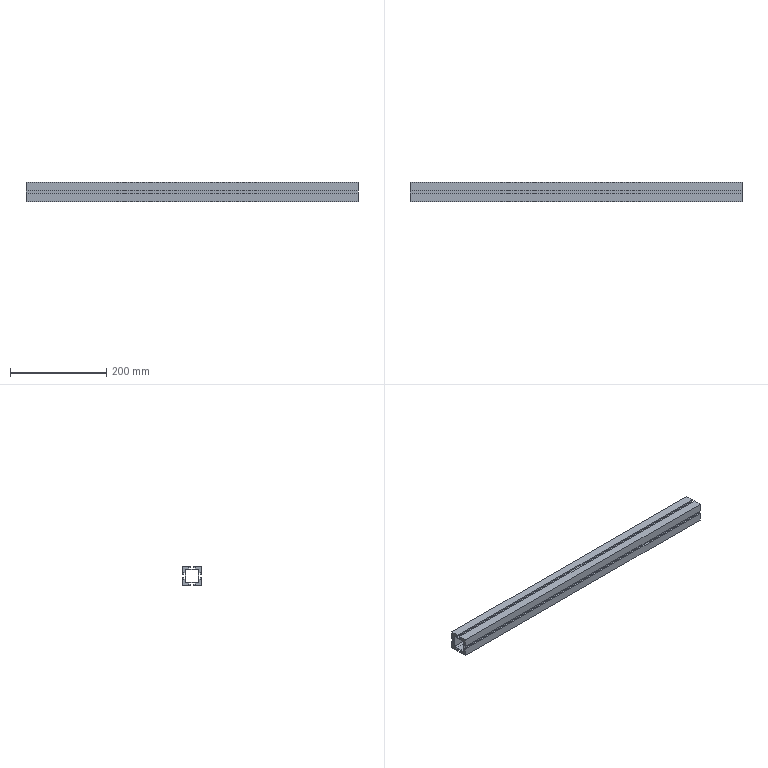Part | SolidWorks | features Extrusion 1 | 1 solid | 42 faces | box 690 x 40 x 40 mm | volume 480240 mm3 | plane 42
STEP:
#1=CARTESIAN_POINT('',(690.,3.,-20.));
#2=VERTEX_POINT('',#1);
#3=CARTESIAN_POINT('',(690.,20.,-20.));
#4=VERTEX_POINT('',#3);
#5=CARTESIAN_POINT('',(690.,3.,-20.));
#6=DIRECTION('',(0.,1.,0.));
#7=VECTOR('',#6,1000.);
#8=LINE('',#5,#7);
#9=EDGE_CURVE('',#2,#4,#8,.T.);
#10=ORIENTED_EDGE('',*,*,#9,.T.);
#11=CARTESIAN_POINT('',(690.,20.,-3.));
#12=VERTEX_POINT('',#11);
#13=CARTESIAN_POINT('',(690.,20.,-3.));
#14=DIRECTION('',(0.,0.,1.));
#15=VECTOR('',#14,1000.);
#16=LINE('',#13,#15);
#17=EDGE_CURVE('',#4,#12,#16,.T.);
#18=ORIENTED_EDGE('',*,*,#17,.T.);
#19=CARTESIAN_POINT('',(690.,17.,-3.));
#20=VERTEX_POINT('',#19);
#21=CARTESIAN_POINT('',(690.,20.,-3.));
#22=DIRECTION('',(0.,-1.,0.));
#23=VECTOR('',#22,1000.);
#24=LINE('',#21,#23);
#25=EDGE_CURVE('',#12,#20,#24,.T.);
#26=ORIENTED_EDGE('',*,*,#25,.T.);
#27=CARTESIAN_POINT('',(690.,17.,-6.5));
#28=VERTEX_POINT('',#27);
#29=CARTESIAN_POINT('',(690.,17.,-3.));
#30=DIRECTION('',(0.,0.,-1.));
#31=VECTOR('',#30,1000.);
#32=LINE('',#29,#31);
#33=EDGE_CURVE('',#20,#28,#32,.T.);
#34=ORIENTED_EDGE('',*,*,#33,.T.);
#35=CARTESIAN_POINT('',(690.,14.,-6.5));
#36=VERTEX_POINT('',#35);
#37=CARTESIAN_POINT('',(690.,17.,-6.5));
#38=DIRECTION('',(0.,-1.,0.));
#39=VECTOR('',#38,1000.);
#40=LINE('',#37,#39);
#41=EDGE_CURVE('',#28,#36,#40,.T.);
#42=ORIENTED_EDGE('',*,*,#41,.T.);
#43=CARTESIAN_POINT('',(690.,14.,6.5));
#44=VERTEX_POINT('',#43);
#45=CARTESIAN_POINT('',(690.,14.,6.5));
#46=DIRECTION('',(0.,0.,1.));
#47=VECTOR('',#46,1000.);
#48=LINE('',#45,#47);
#49=EDGE_CURVE('',#36,#44,#48,.T.);
#50=ORIENTED_EDGE('',*,*,#49,.T.);
#51=CARTESIAN_POINT('',(690.,17.,6.5));
#52=VERTEX_POINT('',#51);
#53=CARTESIAN_POINT('',(690.,17.,6.5));
#54=DIRECTION('',(0.,1.,0.));
#55=VECTOR('',#54,1000.);
#56=LINE('',#53,#55);
#57=EDGE_CURVE('',#44,#52,#56,.T.);
#58=ORIENTED_EDGE('',*,*,#57,.T.);
#59=CARTESIAN_POINT('',(690.,17.,3.));
#60=VERTEX_POINT('',#59);
#61=CARTESIAN_POINT('',(690.,17.,6.5));
#62=DIRECTION('',(0.,0.,-1.));
#63=VECTOR('',#62,1000.);
#64=LINE('',#61,#63);
#65=EDGE_CURVE('',#52,#60,#64,.T.);
#66=ORIENTED_EDGE('',*,*,#65,.T.);
#67=CARTESIAN_POINT('',(690.,20.,3.));
#68=VERTEX_POINT('',#67);
#69=CARTESIAN_POINT('',(690.,20.,3.));
#70=DIRECTION('',(0.,1.,0.));
#71=VECTOR('',#70,1000.);
#72=LINE('',#69,#71);
#73=EDGE_CURVE('',#60,#68,#72,.T.);
#74=ORIENTED_EDGE('',*,*,#73,.T.);
#75=CARTESIAN_POINT('',(690.,20.,20.));
#76=VERTEX_POINT('',#75);
#77=CARTESIAN_POINT('',(690.,20.,20.));
#78=DIRECTION('',(0.,0.,1.));
#79=VECTOR('',#78,1000.);
#80=LINE('',#77,#79);
#81=EDGE_CURVE('',#68,#76,#80,.T.);
#82=ORIENTED_EDGE('',*,*,#81,.T.);
#83=CARTESIAN_POINT('',(690.,3.,20.));
#84=VERTEX_POINT('',#83);
#85=CARTESIAN_POINT('',(690.,3.,20.));
#86=DIRECTION('',(0.,-1.,0.));
#87=VECTOR('',#86,1000.);
#88=LINE('',#85,#87);
#89=EDGE_CURVE('',#76,#84,#88,.T.);
#90=ORIENTED_EDGE('',*,*,#89,.T.);
#91=CARTESIAN_POINT('',(690.,3.,17.));
#92=VERTEX_POINT('',#91);
#93=CARTESIAN_POINT('',(690.,3.,17.));
#94=DIRECTION('',(0.,0.,-1.));
#95=VECTOR('',#94,1000.);
#96=LINE('',#93,#95);
#97=EDGE_CURVE('',#84,#92,#96,.T.);
#98=ORIENTED_EDGE('',*,*,#97,.T.);
#99=CARTESIAN_POINT('',(690.,6.5,17.));
#100=VERTEX_POINT('',#99);
#101=CARTESIAN_POINT('',(690.,3.,17.));
#102=DIRECTION('',(0.,1.,0.));
#103=VECTOR('',#102,1000.);
#104=LINE('',#101,#103);
#105=EDGE_CURVE('',#92,#100,#104,.T.);
#106=ORIENTED_EDGE('',*,*,#105,.T.);
#107=CARTESIAN_POINT('',(690.,6.5,14.));
#108=VERTEX_POINT('',#107);
#109=CARTESIAN_POINT('',(690.,6.5,14.));
#110=DIRECTION('',(0.,0.,-1.));
#111=VECTOR('',#110,1000.);
#112=LINE('',#109,#111);
#113=EDGE_CURVE('',#100,#108,#112,.T.);
#114=ORIENTED_EDGE('',*,*,#113,.T.);
#115=CARTESIAN_POINT('',(690.,-6.5,14.));
#116=VERTEX_POINT('',#115);
#117=CARTESIAN_POINT('',(690.,-6.5,14.));
#118=DIRECTION('',(0.,-1.,0.));
#119=VECTOR('',#118,1000.);
#120=LINE('',#117,#119);
#121=EDGE_CURVE('',#108,#116,#120,.T.);
#122=ORIENTED_EDGE('',*,*,#121,.T.);
#123=CARTESIAN_POINT('',(690.,-6.5,17.));
#124=VERTEX_POINT('',#123);
#125=CARTESIAN_POINT('',(690.,-6.5,14.));
#126=DIRECTION('',(0.,0.,1.));
#127=VECTOR('',#126,1000.);
#128=LINE('',#125,#127);
#129=EDGE_CURVE('',#116,#124,#128,.T.);
#130=ORIENTED_EDGE('',*,*,#129,.T.);
#131=CARTESIAN_POINT('',(690.,-3.,17.));
#132=VERTEX_POINT('',#131);
#133=CARTESIAN_POINT('',(690.,-6.5,17.));
#134=DIRECTION('',(0.,1.,0.));
#135=VECTOR('',#134,1000.);
#136=LINE('',#133,#135);
#137=EDGE_CURVE('',#124,#132,#136,.T.);
#138=ORIENTED_EDGE('',*,*,#137,.T.);
#139=CARTESIAN_POINT('',(690.,-3.,20.));
#140=VERTEX_POINT('',#139);
#141=CARTESIAN_POINT('',(690.,-3.,17.));
#142=DIRECTION('',(0.,0.,1.));
#143=VECTOR('',#142,1000.);
#144=LINE('',#141,#143);
#145=EDGE_CURVE('',#132,#140,#144,.T.);
#146=ORIENTED_EDGE('',*,*,#145,.T.);
#147=CARTESIAN_POINT('',(690.,-20.,20.));
#148=VERTEX_POINT('',#147);
#149=CARTESIAN_POINT('',(690.,-20.,20.));
#150=DIRECTION('',(0.,-1.,0.));
#151=VECTOR('',#150,1000.);
#152=LINE('',#149,#151);
#153=EDGE_CURVE('',#140,#148,#152,.T.);
#154=ORIENTED_EDGE('',*,*,#153,.T.);
#155=CARTESIAN_POINT('',(690.,-20.,3.));
#156=VERTEX_POINT('',#155);
#157=CARTESIAN_POINT('',(690.,-20.,20.));
#158=DIRECTION('',(0.,0.,-1.));
#159=VECTOR('',#158,1000.);
#160=LINE('',#157,#159);
#161=EDGE_CURVE('',#148,#156,#160,.T.);
#162=ORIENTED_EDGE('',*,*,#161,.T.);
#163=CARTESIAN_POINT('',(690.,-17.,3.));
#164=VERTEX_POINT('',#163);
#165=CARTESIAN_POINT('',(690.,-20.,3.));
#166=DIRECTION('',(0.,1.,0.));
#167=VECTOR('',#166,1000.);
#168=LINE('',#165,#167);
#169=EDGE_CURVE('',#156,#164,#168,.T.);
#170=ORIENTED_EDGE('',*,*,#169,.T.);
#171=CARTESIAN_POINT('',(690.,-17.,6.5));
#172=VERTEX_POINT('',#171);
#173=CARTESIAN_POINT('',(690.,-17.,6.5));
#174=DIRECTION('',(0.,0.,1.));
#175=VECTOR('',#174,1000.);
#176=LINE('',#173,#175);
#177=EDGE_CURVE('',#164,#172,#176,.T.);
#178=ORIENTED_EDGE('',*,*,#177,.T.);
#179=CARTESIAN_POINT('',(690.,-14.,6.5));
#180=VERTEX_POINT('',#179);
#181=CARTESIAN_POINT('',(690.,-17.,6.5));
#182=DIRECTION('',(0.,1.,0.));
#183=VECTOR('',#182,1000.);
#184=LINE('',#181,#183);
#185=EDGE_CURVE('',#172,#180,#184,.T.);
#186=ORIENTED_EDGE('',*,*,#185,.T.);
#187=CARTESIAN_POINT('',(690.,-14.,-6.5));
#188=VERTEX_POINT('',#187);
#189=CARTESIAN_POINT('',(690.,-14.,6.5));
#190=DIRECTION('',(0.,0.,-1.));
#191=VECTOR('',#190,1000.);
#192=LINE('',#189,#191);
#193=EDGE_CURVE('',#180,#188,#192,.T.);
#194=ORIENTED_EDGE('',*,*,#193,.T.);
#195=CARTESIAN_POINT('',(690.,-17.,-6.5));
#196=VERTEX_POINT('',#195);
#197=CARTESIAN_POINT('',(690.,-17.,-6.5));
#198=DIRECTION('',(0.,-1.,0.));
#199=VECTOR('',#198,1000.);
#200=LINE('',#197,#199);
#201=EDGE_CURVE('',#188,#196,#200,.T.);
#202=ORIENTED_EDGE('',*,*,#201,.T.);
#203=CARTESIAN_POINT('',(690.,-17.,-3.));
#204=VERTEX_POINT('',#203);
#205=CARTESIAN_POINT('',(690.,-17.,-3.));
#206=DIRECTION('',(0.,0.,1.));
#207=VECTOR('',#206,1000.);
#208=LINE('',#205,#207);
#209=EDGE_CURVE('',#196,#204,#208,.T.);
#210=ORIENTED_EDGE('',*,*,#209,.T.);
#211=CARTESIAN_POINT('',(690.,-20.,-3.));
#212=VERTEX_POINT('',#211);
#213=CARTESIAN_POINT('',(690.,-20.,-3.));
#214=DIRECTION('',(0.,-1.,0.));
#215=VECTOR('',#214,1000.);
#216=LINE('',#213,#215);
#217=EDGE_CURVE('',#204,#212,#216,.T.);
#218=ORIENTED_EDGE('',*,*,#217,.T.);
#219=CARTESIAN_POINT('',(690.,-20.,-20.));
#220=VERTEX_POINT('',#219);
#221=CARTESIAN_POINT('',(690.,-20.,-3.));
#222=DIRECTION('',(0.,0.,-1.));
#223=VECTOR('',#222,1000.);
#224=LINE('',#221,#223);
#225=EDGE_CURVE('',#212,#220,#224,.T.);
#226=ORIENTED_EDGE('',*,*,#225,.T.);
#227=CARTESIAN_POINT('',(690.,-3.,-20.));
#228=VERTEX_POINT('',#227);
#229=CARTESIAN_POINT('',(690.,-20.,-20.));
#230=DIRECTION('',(0.,1.,0.));
#231=VECTOR('',#230,1000.);
#232=LINE('',#229,#231);
#233=EDGE_CURVE('',#220,#228,#232,.T.);
#234=ORIENTED_EDGE('',*,*,#233,.T.);
#235=CARTESIAN_POINT('',(690.,-3.,-17.));
#236=VERTEX_POINT('',#235);
#237=CARTESIAN_POINT('',(690.,-3.,-17.));
#238=DIRECTION('',(0.,0.,1.));
#239=VECTOR('',#238,1000.);
#240=LINE('',#237,#239);
#241=EDGE_CURVE('',#228,#236,#240,.T.);
#242=ORIENTED_EDGE('',*,*,#241,.T.);
#243=CARTESIAN_POINT('',(690.,-6.5,-17.));
#244=VERTEX_POINT('',#243);
#245=CARTESIAN_POINT('',(690.,-6.5,-17.));
#246=DIRECTION('',(0.,-1.,0.));
#247=VECTOR('',#246,1000.);
#248=LINE('',#245,#247);
#249=EDGE_CURVE('',#236,#244,#248,.T.);
#250=ORIENTED_EDGE('',*,*,#249,.T.);
#251=CARTESIAN_POINT('',(690.,-6.5,-14.));
#252=VERTEX_POINT('',#251);
#253=CARTESIAN_POINT('',(690.,-6.5,-14.));
#254=DIRECTION('',(0.,0.,1.));
#255=VECTOR('',#254,1000.);
#256=LINE('',#253,#255);
#257=EDGE_CURVE('',#244,#252,#256,.T.);
#258=ORIENTED_EDGE('',*,*,#257,.T.);
#259=CARTESIAN_POINT('',(690.,6.5,-14.));
#260=VERTEX_POINT('',#259);
#261=CARTESIAN_POINT('',(690.,-6.5,-14.));
#262=DIRECTION('',(0.,1.,0.));
#263=VECTOR('',#262,1000.);
#264=LINE('',#261,#263);
#265=EDGE_CURVE('',#252,#260,#264,.T.);
#266=ORIENTED_EDGE('',*,*,#265,.T.);
#267=CARTESIAN_POINT('',(690.,6.5,-17.));
#268=VERTEX_POINT('',#267);
#269=CARTESIAN_POINT('',(690.,6.5,-14.));
#270=DIRECTION('',(0.,0.,-1.));
#271=VECTOR('',#270,1000.);
#272=LINE('',#269,#271);
#273=EDGE_CURVE('',#260,#268,#272,.T.);
#274=ORIENTED_EDGE('',*,*,#273,.T.);
#275=CARTESIAN_POINT('',(690.,3.,-17.));
#276=VERTEX_POINT('',#275);
#277=CARTESIAN_POINT('',(690.,3.,-17.));
#278=DIRECTION('',(0.,-1.,0.));
#279=VECTOR('',#278,1000.);
#280=LINE('',#277,#279);
#281=EDGE_CURVE('',#268,#276,#280,.T.);
#282=ORIENTED_EDGE('',*,*,#281,.T.);
#283=CARTESIAN_POINT('',(690.,3.,-17.));
#284=DIRECTION('',(0.,0.,-1.));
#285=VECTOR('',#284,1000.);
#286=LINE('',#283,#285);
#287=EDGE_CURVE('',#276,#2,#286,.T.);
#288=ORIENTED_EDGE('',*,*,#287,.T.);
#289=EDGE_LOOP('',(#10,#18,#26,#34,#42,#50,#58,#66,#74,#82,#90,#98,#106,#114,#122,#130,#138,#146,#154,#162,#170,#178,#186,#194,#202,#210,#218,#226,#234,#242,#250,#258,#266,#274,#282,#288));
#290=FACE_OUTER_BOUND('',#289,.T.);
#291=CARTESIAN_POINT('',(690.,-13.,-13.));
#292=VERTEX_POINT('',#291);
#293=CARTESIAN_POINT('',(690.,13.,-13.));
#294=VERTEX_POINT('',#293);
#295=CARTESIAN_POINT('',(690.,-13.,-13.));
#296=DIRECTION('',(0.,1.,0.));
#297=VECTOR('',#296,1000.);
#298=LINE('',#295,#297);
#299=EDGE_CURVE('',#292,#294,#298,.T.);
#300=ORIENTED_EDGE('',*,*,#299,.F.);
#301=CARTESIAN_POINT('',(690.,-13.,13.));
#302=VERTEX_POINT('',#301);
#303=CARTESIAN_POINT('',(690.,-13.,13.));
#304=DIRECTION('',(0.,0.,-1.));
#305=VECTOR('',#304,1000.);
#306=LINE('',#303,#305);
#307=EDGE_CURVE('',#302,#292,#306,.T.);
#308=ORIENTED_EDGE('',*,*,#307,.F.);
#309=CARTESIAN_POINT('',(690.,13.,13.));
#310=VERTEX_POINT('',#309);
#311=CARTESIAN_POINT('',(690.,-13.,13.));
#312=DIRECTION('',(0.,-1.,0.));
#313=VECTOR('',#312,1000.);
#314=LINE('',#311,#313);
#315=EDGE_CURVE('',#310,#302,#314,.T.);
#316=ORIENTED_EDGE('',*,*,#315,.F.);
#317=CARTESIAN_POINT('',(690.,13.,13.));
#318=DIRECTION('',(0.,0.,1.));
#319=VECTOR('',#318,1000.);
#320=LINE('',#317,#319);
#321=EDGE_CURVE('',#294,#310,#320,.T.);
#322=ORIENTED_EDGE('',*,*,#321,.F.);
#323=EDGE_LOOP('',(#300,#308,#316,#322));
#324=FACE_BOUND('',#323,.T.);
#325=CARTESIAN_POINT('',(690.,20.,-20.));
#326=DIRECTION('',(-1.,0.,0.));
#327=DIRECTION('',(0.,0.,1.));
#328=AXIS2_PLACEMENT_3D('',#325,#326,#327);
#329=PLANE('',#328);
#330=ADVANCED_FACE('',(#290,#324),#329,.F.);
#331=CARTESIAN_POINT('',(0.,3.,-20.));
#332=VERTEX_POINT('',#331);
#333=CARTESIAN_POINT('',(0.,20.,-20.));
#334=VERTEX_POINT('',#333);
#335=CARTESIAN_POINT('',(0.,3.,-20.));
#336=DIRECTION('',(0.,1.,0.));
#337=VECTOR('',#336,1000.);
#338=LINE('',#335,#337);
#339=EDGE_CURVE('',#332,#334,#338,.T.);
#340=ORIENTED_EDGE('',*,*,#339,.F.);
#341=CARTESIAN_POINT('',(0.,3.,-17.));
#342=VERTEX_POINT('',#341);
#343=CARTESIAN_POINT('',(0.,3.,-17.));
#344=DIRECTION('',(0.,0.,-1.));
#345=VECTOR('',#344,1000.);
#346=LINE('',#343,#345);
#347=EDGE_CURVE('',#342,#332,#346,.T.);
#348=ORIENTED_EDGE('',*,*,#347,.F.);
#349=CARTESIAN_POINT('',(0.,6.5,-17.));
#350=VERTEX_POINT('',#349);
#351=CARTESIAN_POINT('',(0.,3.,-17.));
#352=DIRECTION('',(0.,-1.,0.));
#353=VECTOR('',#352,1000.);
#354=LINE('',#351,#353);
#355=EDGE_CURVE('',#350,#342,#354,.T.);
#356=ORIENTED_EDGE('',*,*,#355,.F.);
#357=CARTESIAN_POINT('',(0.,6.5,-14.));
#358=VERTEX_POINT('',#357);
#359=CARTESIAN_POINT('',(0.,6.5,-14.));
#360=DIRECTION('',(0.,0.,-1.));
#361=VECTOR('',#360,1000.);
#362=LINE('',#359,#361);
#363=EDGE_CURVE('',#358,#350,#362,.T.);
#364=ORIENTED_EDGE('',*,*,#363,.F.);
#365=CARTESIAN_POINT('',(0.,-6.5,-14.));
#366=VERTEX_POINT('',#365);
#367=CARTESIAN_POINT('',(0.,-6.5,-14.));
#368=DIRECTION('',(0.,1.,0.));
#369=VECTOR('',#368,1000.);
#370=LINE('',#367,#369);
#371=EDGE_CURVE('',#366,#358,#370,.T.);
#372=ORIENTED_EDGE('',*,*,#371,.F.);
#373=CARTESIAN_POINT('',(0.,-6.5,-17.));
#374=VERTEX_POINT('',#373);
#375=CARTESIAN_POINT('',(0.,-6.5,-14.));
#376=DIRECTION('',(0.,0.,1.));
#377=VECTOR('',#376,1000.);
#378=LINE('',#375,#377);
#379=EDGE_CURVE('',#374,#366,#378,.T.);
#380=ORIENTED_EDGE('',*,*,#379,.F.);
#381=CARTESIAN_POINT('',(0.,-3.,-17.));
#382=VERTEX_POINT('',#381);
#383=CARTESIAN_POINT('',(0.,-6.5,-17.));
#384=DIRECTION('',(0.,-1.,0.));
#385=VECTOR('',#384,1000.);
#386=LINE('',#383,#385);
#387=EDGE_CURVE('',#382,#374,#386,.T.);
#388=ORIENTED_EDGE('',*,*,#387,.F.);
#389=CARTESIAN_POINT('',(0.,-3.,-20.));
#390=VERTEX_POINT('',#389);
#391=CARTESIAN_POINT('',(0.,-3.,-17.));
#392=DIRECTION('',(0.,0.,1.));
#393=VECTOR('',#392,1000.);
#394=LINE('',#391,#393);
#395=EDGE_CURVE('',#390,#382,#394,.T.);
#396=ORIENTED_EDGE('',*,*,#395,.F.);
#397=CARTESIAN_POINT('',(0.,-20.,-20.));
#398=VERTEX_POINT('',#397);
#399=CARTESIAN_POINT('',(0.,-20.,-20.));
#400=DIRECTION('',(0.,1.,0.));
#401=VECTOR('',#400,1000.);
#402=LINE('',#399,#401);
#403=EDGE_CURVE('',#398,#390,#402,.T.);
#404=ORIENTED_EDGE('',*,*,#403,.F.);
#405=CARTESIAN_POINT('',(0.,-20.,-3.));
#406=VERTEX_POINT('',#405);
#407=CARTESIAN_POINT('',(0.,-20.,-3.));
#408=DIRECTION('',(0.,0.,-1.));
#409=VECTOR('',#408,1000.);
#410=LINE('',#407,#409);
#411=EDGE_CURVE('',#406,#398,#410,.T.);
#412=ORIENTED_EDGE('',*,*,#411,.F.);
#413=CARTESIAN_POINT('',(0.,-17.,-3.));
#414=VERTEX_POINT('',#413);
#415=CARTESIAN_POINT('',(0.,-20.,-3.));
#416=DIRECTION('',(0.,-1.,0.));
#417=VECTOR('',#416,1000.);
#418=LINE('',#415,#417);
#419=EDGE_CURVE('',#414,#406,#418,.T.);
#420=ORIENTED_EDGE('',*,*,#419,.F.);
#421=CARTESIAN_POINT('',(0.,-17.,-6.5));
#422=VERTEX_POINT('',#421);
#423=CARTESIAN_POINT('',(0.,-17.,-3.));
#424=DIRECTION('',(0.,0.,1.));
#425=VECTOR('',#424,1000.);
#426=LINE('',#423,#425);
#427=EDGE_CURVE('',#422,#414,#426,.T.);
#428=ORIENTED_EDGE('',*,*,#427,.F.);
#429=CARTESIAN_POINT('',(0.,-14.,-6.5));
#430=VERTEX_POINT('',#429);
#431=CARTESIAN_POINT('',(0.,-17.,-6.5));
#432=DIRECTION('',(0.,-1.,0.));
#433=VECTOR('',#432,1000.);
#434=LINE('',#431,#433);
#435=EDGE_CURVE('',#430,#422,#434,.T.);
#436=ORIENTED_EDGE('',*,*,#435,.F.);
#437=CARTESIAN_POINT('',(0.,-14.,6.5));
#438=VERTEX_POINT('',#437);
#439=CARTESIAN_POINT('',(0.,-14.,6.5));
#440=DIRECTION('',(0.,0.,-1.));
#441=VECTOR('',#440,1000.);
#442=LINE('',#439,#441);
#443=EDGE_CURVE('',#438,#430,#442,.T.);
#444=ORIENTED_EDGE('',*,*,#443,.F.);
#445=CARTESIAN_POINT('',(0.,-17.,6.5));
#446=VERTEX_POINT('',#445);
#447=CARTESIAN_POINT('',(0.,-17.,6.5));
#448=DIRECTION('',(0.,1.,0.));
#449=VECTOR('',#448,1000.);
#450=LINE('',#447,#449);
#451=EDGE_CURVE('',#446,#438,#450,.T.);
#452=ORIENTED_EDGE('',*,*,#451,.F.);
#453=CARTESIAN_POINT('',(0.,-17.,3.));
#454=VERTEX_POINT('',#453);
#455=CARTESIAN_POINT('',(0.,-17.,6.5));
#456=DIRECTION('',(0.,0.,1.));
#457=VECTOR('',#456,1000.);
#458=LINE('',#455,#457);
#459=EDGE_CURVE('',#454,#446,#458,.T.);
#460=ORIENTED_EDGE('',*,*,#459,.F.);
#461=CARTESIAN_POINT('',(0.,-20.,3.));
#462=VERTEX_POINT('',#461);
#463=CARTESIAN_POINT('',(0.,-20.,3.));
#464=DIRECTION('',(0.,1.,0.));
#465=VECTOR('',#464,1000.);
#466=LINE('',#463,#465);
#467=EDGE_CURVE('',#462,#454,#466,.T.);
#468=ORIENTED_EDGE('',*,*,#467,.F.);
#469=CARTESIAN_POINT('',(0.,-20.,20.));
#470=VERTEX_POINT('',#469);
#471=CARTESIAN_POINT('',(0.,-20.,20.));
#472=DIRECTION('',(0.,0.,-1.));
#473=VECTOR('',#472,1000.);
#474=LINE('',#471,#473);
#475=EDGE_CURVE('',#470,#462,#474,.T.);
#476=ORIENTED_EDGE('',*,*,#475,.F.);
#477=CARTESIAN_POINT('',(0.,-3.,20.));
#478=VERTEX_POINT('',#477);
#479=CARTESIAN_POINT('',(0.,-20.,20.));
#480=DIRECTION('',(0.,-1.,0.));
#481=VECTOR('',#480,1000.);
#482=LINE('',#479,#481);
#483=EDGE_CURVE('',#478,#470,#482,.T.);
#484=ORIENTED_EDGE('',*,*,#483,.F.);
#485=CARTESIAN_POINT('',(0.,-3.,17.));
#486=VERTEX_POINT('',#485);
#487=CARTESIAN_POINT('',(0.,-3.,17.));
#488=DIRECTION('',(0.,0.,1.));
#489=VECTOR('',#488,1000.);
#490=LINE('',#487,#489);
#491=EDGE_CURVE('',#486,#478,#490,.T.);
#492=ORIENTED_EDGE('',*,*,#491,.F.);
#493=CARTESIAN_POINT('',(0.,-6.5,17.));
#494=VERTEX_POINT('',#493);
#495=CARTESIAN_POINT('',(0.,-6.5,17.));
#496=DIRECTION('',(0.,1.,0.));
#497=VECTOR('',#496,1000.);
#498=LINE('',#495,#497);
#499=EDGE_CURVE('',#494,#486,#498,.T.);
#500=ORIENTED_EDGE('',*,*,#499,.F.);
#501=CARTESIAN_POINT('',(0.,-6.5,14.));
#502=VERTEX_POINT('',#501);
#503=CARTESIAN_POINT('',(0.,-6.5,14.));
#504=DIRECTION('',(0.,0.,1.));
#505=VECTOR('',#504,1000.);
#506=LINE('',#503,#505);
#507=EDGE_CURVE('',#502,#494,#506,.T.);
#508=ORIENTED_EDGE('',*,*,#507,.F.);
#509=CARTESIAN_POINT('',(0.,6.5,14.));
#510=VERTEX_POINT('',#509);
#511=CARTESIAN_POINT('',(0.,-6.5,14.));
#512=DIRECTION('',(0.,-1.,0.));
#513=VECTOR('',#512,1000.);
#514=LINE('',#511,#513);
#515=EDGE_CURVE('',#510,#502,#514,.T.);
#516=ORIENTED_EDGE('',*,*,#515,.F.);
#517=CARTESIAN_POINT('',(0.,6.5,17.));
#518=VERTEX_POINT('',#517);
#519=CARTESIAN_POINT('',(0.,6.5,14.));
#520=DIRECTION('',(0.,0.,-1.));
#521=VECTOR('',#520,1000.);
#522=LINE('',#519,#521);
#523=EDGE_CURVE('',#518,#510,#522,.T.);
#524=ORIENTED_EDGE('',*,*,#523,.F.);
#525=CARTESIAN_POINT('',(0.,3.,17.));
#526=VERTEX_POINT('',#525);
#527=CARTESIAN_POINT('',(0.,3.,17.));
#528=DIRECTION('',(0.,1.,0.));
#529=VECTOR('',#528,1000.);
#530=LINE('',#527,#529);
#531=EDGE_CURVE('',#526,#518,#530,.T.);
#532=ORIENTED_EDGE('',*,*,#531,.F.);
#533=CARTESIAN_POINT('',(0.,3.,20.));
#534=VERTEX_POINT('',#533);
#535=CARTESIAN_POINT('',(0.,3.,17.));
#536=DIRECTION('',(0.,0.,-1.));
#537=VECTOR('',#536,1000.);
#538=LINE('',#535,#537);
#539=EDGE_CURVE('',#534,#526,#538,.T.);
#540=ORIENTED_EDGE('',*,*,#539,.F.);
#541=CARTESIAN_POINT('',(0.,20.,20.));
#542=VERTEX_POINT('',#541);
#543=CARTESIAN_POINT('',(0.,3.,20.));
#544=DIRECTION('',(0.,-1.,0.));
#545=VECTOR('',#544,1000.);
#546=LINE('',#543,#545);
#547=EDGE_CURVE('',#542,#534,#546,.T.);
#548=ORIENTED_EDGE('',*,*,#547,.F.);
#549=CARTESIAN_POINT('',(0.,20.,3.));
#550=VERTEX_POINT('',#549);
#551=CARTESIAN_POINT('',(0.,20.,20.));
#552=DIRECTION('',(0.,0.,1.));
#553=VECTOR('',#552,1000.);
#554=LINE('',#551,#553);
#555=EDGE_CURVE('',#550,#542,#554,.T.);
#556=ORIENTED_EDGE('',*,*,#555,.F.);
#557=CARTESIAN_POINT('',(0.,17.,3.));
#558=VERTEX_POINT('',#557);
#559=CARTESIAN_POINT('',(0.,20.,3.));
#560=DIRECTION('',(0.,1.,0.));
#561=VECTOR('',#560,1000.);
#562=LINE('',#559,#561);
#563=EDGE_CURVE('',#558,#550,#562,.T.);
#564=ORIENTED_EDGE('',*,*,#563,.F.);
#565=CARTESIAN_POINT('',(0.,17.,6.5));
#566=VERTEX_POINT('',#565);
#567=CARTESIAN_POINT('',(0.,17.,6.5));
#568=DIRECTION('',(0.,0.,-1.));
#569=VECTOR('',#568,1000.);
#570=LINE('',#567,#569);
#571=EDGE_CURVE('',#566,#558,#570,.T.);
#572=ORIENTED_EDGE('',*,*,#571,.F.);
#573=CARTESIAN_POINT('',(0.,14.,6.5));
#574=VERTEX_POINT('',#573);
#575=CARTESIAN_POINT('',(0.,17.,6.5));
#576=DIRECTION('',(0.,1.,0.));
#577=VECTOR('',#576,1000.);
#578=LINE('',#575,#577);
#579=EDGE_CURVE('',#574,#566,#578,.T.);
#580=ORIENTED_EDGE('',*,*,#579,.F.);
#581=CARTESIAN_POINT('',(0.,14.,-6.5));
#582=VERTEX_POINT('',#581);
#583=CARTESIAN_POINT('',(0.,14.,6.5));
#584=DIRECTION('',(0.,0.,1.));
#585=VECTOR('',#584,1000.);
#586=LINE('',#583,#585);
#587=EDGE_CURVE('',#582,#574,#586,.T.);
#588=ORIENTED_EDGE('',*,*,#587,.F.);
#589=CARTESIAN_POINT('',(0.,17.,-6.5));
#590=VERTEX_POINT('',#589);
#591=CARTESIAN_POINT('',(0.,17.,-6.5));
#592=DIRECTION('',(0.,-1.,0.));
#593=VECTOR('',#592,1000.);
#594=LINE('',#591,#593);
#595=EDGE_CURVE('',#590,#582,#594,.T.);
#596=ORIENTED_EDGE('',*,*,#595,.F.);
#597=CARTESIAN_POINT('',(0.,17.,-3.));
#598=VERTEX_POINT('',#597);
#599=CARTESIAN_POINT('',(0.,17.,-3.));
#600=DIRECTION('',(0.,0.,-1.));
#601=VECTOR('',#600,1000.);
#602=LINE('',#599,#601);
#603=EDGE_CURVE('',#598,#590,#602,.T.);
#604=ORIENTED_EDGE('',*,*,#603,.F.);
#605=CARTESIAN_POINT('',(0.,20.,-3.));
#606=VERTEX_POINT('',#605);
#607=CARTESIAN_POINT('',(0.,20.,-3.));
#608=DIRECTION('',(0.,-1.,0.));
#609=VECTOR('',#608,1000.);
#610=LINE('',#607,#609);
#611=EDGE_CURVE('',#606,#598,#610,.T.);
#612=ORIENTED_EDGE('',*,*,#611,.F.);
#613=CARTESIAN_POINT('',(0.,20.,-3.));
#614=DIRECTION('',(0.,0.,1.));
#615=VECTOR('',#614,1000.);
#616=LINE('',#613,#615);
#617=EDGE_CURVE('',#334,#606,#616,.T.);
#618=ORIENTED_EDGE('',*,*,#617,.F.);
#619=EDGE_LOOP('',(#340,#348,#356,#364,#372,#380,#388,#396,#404,#412,#420,#428,#436,#444,#452,#460,#468,#476,#484,#492,#500,#508,#516,#524,#532,#540,#548,#556,#564,#572,#580,#588,#596,#604,#612,#618));
#620=FACE_OUTER_BOUND('',#619,.T.);
#621=CARTESIAN_POINT('',(0.,-13.,13.));
#622=VERTEX_POINT('',#621);
#623=CARTESIAN_POINT('',(0.,-13.,-13.));
#624=VERTEX_POINT('',#623);
#625=CARTESIAN_POINT('',(0.,-13.,13.));
#626=DIRECTION('',(0.,0.,-1.));
#627=VECTOR('',#626,1000.);
#628=LINE('',#625,#627);
#629=EDGE_CURVE('',#622,#624,#628,.T.);
#630=ORIENTED_EDGE('',*,*,#629,.T.);
#631=CARTESIAN_POINT('',(0.,13.,-13.));
#632=VERTEX_POINT('',#631);
#633=CARTESIAN_POINT('',(0.,-13.,-13.));
#634=DIRECTION('',(0.,1.,0.));
#635=VECTOR('',#634,1000.);
#636=LINE('',#633,#635);
#637=EDGE_CURVE('',#624,#632,#636,.T.);
#638=ORIENTED_EDGE('',*,*,#637,.T.);
#639=CARTESIAN_POINT('',(0.,13.,13.));
#640=VERTEX_POINT('',#639);
#641=CARTESIAN_POINT('',(0.,13.,13.));
#642=DIRECTION('',(0.,0.,1.));
#643=VECTOR('',#642,1000.);
#644=LINE('',#641,#643);
#645=EDGE_CURVE('',#632,#640,#644,.T.);
#646=ORIENTED_EDGE('',*,*,#645,.T.);
#647=CARTESIAN_POINT('',(0.,-13.,13.));
#648=DIRECTION('',(0.,-1.,0.));
#649=VECTOR('',#648,1000.);
#650=LINE('',#647,#649);
#651=EDGE_CURVE('',#640,#622,#650,.T.);
#652=ORIENTED_EDGE('',*,*,#651,.T.);
#653=EDGE_LOOP('',(#630,#638,#646,#652));
#654=FACE_BOUND('',#653,.T.);
#655=CARTESIAN_POINT('',(0.,20.,-20.));
#656=DIRECTION('',(-1.,0.,0.));
#657=DIRECTION('',(0.,0.,1.));
#658=AXIS2_PLACEMENT_3D('',#655,#656,#657);
#659=PLANE('',#658);
#660=ADVANCED_FACE('',(#620,#654),#659,.T.);
#661=ORIENTED_EDGE('',*,*,#339,.T.);
#662=CARTESIAN_POINT('',(690.,20.,-20.));
#663=DIRECTION('',(-1.,0.,0.));
#664=VECTOR('',#663,1000.);
#665=LINE('',#662,#664);
#666=EDGE_CURVE('',#4,#334,#665,.T.);
#667=ORIENTED_EDGE('',*,*,#666,.F.);
#668=ORIENTED_EDGE('',*,*,#9,.F.);
#669=CARTESIAN_POINT('',(690.,3.,-20.));
#670=DIRECTION('',(-1.,0.,0.));
#671=VECTOR('',#670,1000.);
#672=LINE('',#669,#671);
#673=EDGE_CURVE('',#2,#332,#672,.T.);
#674=ORIENTED_EDGE('',*,*,#673,.T.);
#675=EDGE_LOOP('',(#661,#667,#668,#674));
#676=FACE_OUTER_BOUND('',#675,.T.);
#677=CARTESIAN_POINT('',(690.,3.,-20.));
#678=DIRECTION('',(0.,0.,1.));
#679=DIRECTION('',(0.,-1.,0.));
#680=AXIS2_PLACEMENT_3D('',#677,#678,#679);
#681=PLANE('',#680);
#682=ADVANCED_FACE('',(#676),#681,.F.);
#683=ORIENTED_EDGE('',*,*,#617,.T.);
#684=CARTESIAN_POINT('',(690.,20.,-3.));
#685=DIRECTION('',(-1.,0.,0.));
#686=VECTOR('',#685,1000.);
#687=LINE('',#684,#686);
#688=EDGE_CURVE('',#12,#606,#687,.T.);
#689=ORIENTED_EDGE('',*,*,#688,.F.);
#690=ORIENTED_EDGE('',*,*,#17,.F.);
#691=ORIENTED_EDGE('',*,*,#666,.T.);
#692=EDGE_LOOP('',(#683,#689,#690,#691));
#693=FACE_OUTER_BOUND('',#692,.T.);
#694=CARTESIAN_POINT('',(690.,20.,-3.));
#695=DIRECTION('',(0.,-1.,0.));
#696=DIRECTION('',(0.,0.,-1.));
#697=AXIS2_PLACEMENT_3D('',#694,#695,#696);
#698=PLANE('',#697);
#699=ADVANCED_FACE('',(#693),#698,.F.);
#700=ORIENTED_EDGE('',*,*,#611,.T.);
#701=CARTESIAN_POINT('',(690.,17.,-3.));
#702=DIRECTION('',(-1.,0.,0.));
#703=VECTOR('',#702,1000.);
#704=LINE('',#701,#703);
#705=EDGE_CURVE('',#20,#598,#704,.T.);
#706=ORIENTED_EDGE('',*,*,#705,.F.);
#707=ORIENTED_EDGE('',*,*,#25,.F.);
#708=ORIENTED_EDGE('',*,*,#688,.T.);
#709=EDGE_LOOP('',(#700,#706,#707,#708));
#710=FACE_OUTER_BOUND('',#709,.T.);
#711=CARTESIAN_POINT('',(690.,20.,-3.));
#712=DIRECTION('',(0.,0.,-1.));
#713=DIRECTION('',(0.,1.,0.));
#714=AXIS2_PLACEMENT_3D('',#711,#712,#713);
#715=PLANE('',#714);
#716=ADVANCED_FACE('',(#710),#715,.F.);
#717=ORIENTED_EDGE('',*,*,#603,.T.);
#718=CARTESIAN_POINT('',(690.,17.,-6.5));
#719=DIRECTION('',(-1.,0.,0.));
#720=VECTOR('',#719,1000.);
#721=LINE('',#718,#720);
#722=EDGE_CURVE('',#28,#590,#721,.T.);
#723=ORIENTED_EDGE('',*,*,#722,.F.);
#724=ORIENTED_EDGE('',*,*,#33,.F.);
#725=ORIENTED_EDGE('',*,*,#705,.T.);
#726=EDGE_LOOP('',(#717,#723,#724,#725));
#727=FACE_OUTER_BOUND('',#726,.T.);
#728=CARTESIAN_POINT('',(690.,17.,-3.));
#729=DIRECTION('',(0.,1.,0.));
#730=DIRECTION('',(0.,0.,1.));
#731=AXIS2_PLACEMENT_3D('',#728,#729,#730);
#732=PLANE('',#731);
#733=ADVANCED_FACE('',(#727),#732,.F.);
#734=ORIENTED_EDGE('',*,*,#595,.T.);
#735=CARTESIAN_POINT('',(690.,14.,-6.5));
#736=DIRECTION('',(-1.,0.,0.));
#737=VECTOR('',#736,1000.);
#738=LINE('',#735,#737);
#739=EDGE_CURVE('',#36,#582,#738,.T.);
#740=ORIENTED_EDGE('',*,*,#739,.F.);
#741=ORIENTED_EDGE('',*,*,#41,.F.);
#742=ORIENTED_EDGE('',*,*,#722,.T.);
#743=EDGE_LOOP('',(#734,#740,#741,#742));
#744=FACE_OUTER_BOUND('',#743,.T.);
#745=CARTESIAN_POINT('',(690.,17.,-6.5));
#746=DIRECTION('',(0.,0.,-1.));
#747=DIRECTION('',(-1.,0.,0.));
#748=AXIS2_PLACEMENT_3D('',#745,#746,#747);
#749=PLANE('',#748);
#750=ADVANCED_FACE('',(#744),#749,.F.);
#751=ORIENTED_EDGE('',*,*,#587,.T.);
#752=CARTESIAN_POINT('',(690.,14.,6.5));
#753=DIRECTION('',(-1.,0.,0.));
#754=VECTOR('',#753,1000.);
#755=LINE('',#752,#754);
#756=EDGE_CURVE('',#44,#574,#755,.T.);
#757=ORIENTED_EDGE('',*,*,#756,.F.);
#758=ORIENTED_EDGE('',*,*,#49,.F.);
#759=ORIENTED_EDGE('',*,*,#739,.T.);
#760=EDGE_LOOP('',(#751,#757,#758,#759));
#761=FACE_OUTER_BOUND('',#760,.T.);
#762=CARTESIAN_POINT('',(690.,14.,6.5));
#763=DIRECTION('',(0.,-1.,0.));
#764=DIRECTION('',(0.,0.,-1.));
#765=AXIS2_PLACEMENT_3D('',#762,#763,#764);
#766=PLANE('',#765);
#767=ADVANCED_FACE('',(#761),#766,.F.);
#768=ORIENTED_EDGE('',*,*,#579,.T.);
#769=CARTESIAN_POINT('',(690.,17.,6.5));
#770=DIRECTION('',(-1.,0.,0.));
#771=VECTOR('',#770,1000.);
#772=LINE('',#769,#771);
#773=EDGE_CURVE('',#52,#566,#772,.T.);
#774=ORIENTED_EDGE('',*,*,#773,.F.);
#775=ORIENTED_EDGE('',*,*,#57,.F.);
#776=ORIENTED_EDGE('',*,*,#756,.T.);
#777=EDGE_LOOP('',(#768,#774,#775,#776));
#778=FACE_OUTER_BOUND('',#777,.T.);
#779=CARTESIAN_POINT('',(690.,17.,6.5));
#780=DIRECTION('',(0.,0.,1.));
#781=DIRECTION('',(1.,0.,0.));
#782=AXIS2_PLACEMENT_3D('',#779,#780,#781);
#783=PLANE('',#782);
#784=ADVANCED_FACE('',(#778),#783,.F.);
#785=ORIENTED_EDGE('',*,*,#571,.T.);
#786=CARTESIAN_POINT('',(690.,17.,3.));
#787=DIRECTION('',(-1.,0.,0.));
#788=VECTOR('',#787,1000.);
#789=LINE('',#786,#788);
#790=EDGE_CURVE('',#60,#558,#789,.T.);
#791=ORIENTED_EDGE('',*,*,#790,.F.);
#792=ORIENTED_EDGE('',*,*,#65,.F.);
#793=ORIENTED_EDGE('',*,*,#773,.T.);
#794=EDGE_LOOP('',(#785,#791,#792,#793));
#795=FACE_OUTER_BOUND('',#794,.T.);
#796=CARTESIAN_POINT('',(690.,17.,6.5));
#797=DIRECTION('',(0.,1.,0.));
#798=DIRECTION('',(0.,0.,1.));
#799=AXIS2_PLACEMENT_3D('',#796,#797,#798);
#800=PLANE('',#799);
#801=ADVANCED_FACE('',(#795),#800,.F.);
#802=ORIENTED_EDGE('',*,*,#563,.T.);
#803=CARTESIAN_POINT('',(690.,20.,3.));
#804=DIRECTION('',(-1.,0.,0.));
#805=VECTOR('',#804,1000.);
#806=LINE('',#803,#805);
#807=EDGE_CURVE('',#68,#550,#806,.T.);
#808=ORIENTED_EDGE('',*,*,#807,.F.);
#809=ORIENTED_EDGE('',*,*,#73,.F.);
#810=ORIENTED_EDGE('',*,*,#790,.T.);
#811=EDGE_LOOP('',(#802,#808,#809,#810));
#812=FACE_OUTER_BOUND('',#811,.T.);
#813=CARTESIAN_POINT('',(690.,20.,3.));
#814=DIRECTION('',(0.,0.,1.));
#815=DIRECTION('',(0.,-1.,0.));
#816=AXIS2_PLACEMENT_3D('',#813,#814,#815);
#817=PLANE('',#816);
#818=ADVANCED_FACE('',(#812),#817,.F.);
#819=ORIENTED_EDGE('',*,*,#555,.T.);
#820=CARTESIAN_POINT('',(690.,20.,20.));
#821=DIRECTION('',(-1.,0.,0.));
#822=VECTOR('',#821,1000.);
#823=LINE('',#820,#822);
#824=EDGE_CURVE('',#76,#542,#823,.T.);
#825=ORIENTED_EDGE('',*,*,#824,.F.);
#826=ORIENTED_EDGE('',*,*,#81,.F.);
#827=ORIENTED_EDGE('',*,*,#807,.T.);
#828=EDGE_LOOP('',(#819,#825,#826,#827));
#829=FACE_OUTER_BOUND('',#828,.T.);
#830=CARTESIAN_POINT('',(690.,20.,20.));
#831=DIRECTION('',(0.,-1.,0.));
#832=DIRECTION('',(0.,0.,-1.));
#833=AXIS2_PLACEMENT_3D('',#830,#831,#832);
#834=PLANE('',#833);
#835=ADVANCED_FACE('',(#829),#834,.F.);
#836=ORIENTED_EDGE('',*,*,#547,.T.);
#837=CARTESIAN_POINT('',(690.,3.,20.));
#838=DIRECTION('',(-1.,0.,0.));
#839=VECTOR('',#838,1000.);
#840=LINE('',#837,#839);
#841=EDGE_CURVE('',#84,#534,#840,.T.);
#842=ORIENTED_EDGE('',*,*,#841,.F.);
#843=ORIENTED_EDGE('',*,*,#89,.F.);
#844=ORIENTED_EDGE('',*,*,#824,.T.);
#845=EDGE_LOOP('',(#836,#842,#843,#844));
#846=FACE_OUTER_BOUND('',#845,.T.);
#847=CARTESIAN_POINT('',(690.,3.,20.));
#848=DIRECTION('',(0.,0.,-1.));
#849=DIRECTION('',(0.,1.,0.));
#850=AXIS2_PLACEMENT_3D('',#847,#848,#849);
#851=PLANE('',#850);
#852=ADVANCED_FACE('',(#846),#851,.F.);
#853=ORIENTED_EDGE('',*,*,#539,.T.);
#854=CARTESIAN_POINT('',(690.,3.,17.));
#855=DIRECTION('',(-1.,0.,0.));
#856=VECTOR('',#855,1000.);
#857=LINE('',#854,#856);
#858=EDGE_CURVE('',#92,#526,#857,.T.);
#859=ORIENTED_EDGE('',*,*,#858,.F.);
#860=ORIENTED_EDGE('',*,*,#97,.F.);
#861=ORIENTED_EDGE('',*,*,#841,.T.);
#862=EDGE_LOOP('',(#853,#859,#860,#861));
#863=FACE_OUTER_BOUND('',#862,.T.);
#864=CARTESIAN_POINT('',(690.,3.,17.));
#865=DIRECTION('',(0.,1.,0.));
#866=DIRECTION('',(0.,0.,1.));
#867=AXIS2_PLACEMENT_3D('',#864,#865,#866);
#868=PLANE('',#867);
#869=ADVANCED_FACE('',(#863),#868,.F.);
#870=ORIENTED_EDGE('',*,*,#531,.T.);
#871=CARTESIAN_POINT('',(690.,6.5,17.));
#872=DIRECTION('',(-1.,0.,0.));
#873=VECTOR('',#872,1000.);
#874=LINE('',#871,#873);
#875=EDGE_CURVE('',#100,#518,#874,.T.);
#876=ORIENTED_EDGE('',*,*,#875,.F.);
#877=ORIENTED_EDGE('',*,*,#105,.F.);
#878=ORIENTED_EDGE('',*,*,#858,.T.);
#879=EDGE_LOOP('',(#870,#876,#877,#878));
#880=FACE_OUTER_BOUND('',#879,.T.);
#881=CARTESIAN_POINT('',(690.,3.,17.));
#882=DIRECTION('',(0.,0.,1.));
#883=DIRECTION('',(1.,0.,0.));
#884=AXIS2_PLACEMENT_3D('',#881,#882,#883);
#885=PLANE('',#884);
#886=ADVANCED_FACE('',(#880),#885,.F.);
#887=ORIENTED_EDGE('',*,*,#523,.T.);
#888=CARTESIAN_POINT('',(690.,6.5,14.));
#889=DIRECTION('',(-1.,0.,0.));
#890=VECTOR('',#889,1000.);
#891=LINE('',#888,#890);
#892=EDGE_CURVE('',#108,#510,#891,.T.);
#893=ORIENTED_EDGE('',*,*,#892,.F.);
#894=ORIENTED_EDGE('',*,*,#113,.F.);
#895=ORIENTED_EDGE('',*,*,#875,.T.);
#896=EDGE_LOOP('',(#887,#893,#894,#895));
#897=FACE_OUTER_BOUND('',#896,.T.);
#898=CARTESIAN_POINT('',(690.,6.5,14.));
#899=DIRECTION('',(0.,1.,0.));
#900=DIRECTION('',(0.,0.,1.));
#901=AXIS2_PLACEMENT_3D('',#898,#899,#900);
#902=PLANE('',#901);
#903=ADVANCED_FACE('',(#897),#902,.F.);
#904=ORIENTED_EDGE('',*,*,#515,.T.);
#905=CARTESIAN_POINT('',(690.,-6.5,14.));
#906=DIRECTION('',(-1.,0.,0.));
#907=VECTOR('',#906,1000.);
#908=LINE('',#905,#907);
#909=EDGE_CURVE('',#116,#502,#908,.T.);
#910=ORIENTED_EDGE('',*,*,#909,.F.);
#911=ORIENTED_EDGE('',*,*,#121,.F.);
#912=ORIENTED_EDGE('',*,*,#892,.T.);
#913=EDGE_LOOP('',(#904,#910,#911,#912));
#914=FACE_OUTER_BOUND('',#913,.T.);
#915=CARTESIAN_POINT('',(690.,-6.5,14.));
#916=DIRECTION('',(0.,0.,-1.));
#917=DIRECTION('',(-1.,0.,0.));
#918=AXIS2_PLACEMENT_3D('',#915,#916,#917);
#919=PLANE('',#918);
#920=ADVANCED_FACE('',(#914),#919,.F.);
#921=ORIENTED_EDGE('',*,*,#507,.T.);
#922=CARTESIAN_POINT('',(690.,-6.5,17.));
#923=DIRECTION('',(-1.,0.,0.));
#924=VECTOR('',#923,1000.);
#925=LINE('',#922,#924);
#926=EDGE_CURVE('',#124,#494,#925,.T.);
#927=ORIENTED_EDGE('',*,*,#926,.F.);
#928=ORIENTED_EDGE('',*,*,#129,.F.);
#929=ORIENTED_EDGE('',*,*,#909,.T.);
#930=EDGE_LOOP('',(#921,#927,#928,#929));
#931=FACE_OUTER_BOUND('',#930,.T.);
#932=CARTESIAN_POINT('',(690.,-6.5,14.));
#933=DIRECTION('',(0.,-1.,0.));
#934=DIRECTION('',(0.,0.,-1.));
#935=AXIS2_PLACEMENT_3D('',#932,#933,#934);
#936=PLANE('',#935);
#937=ADVANCED_FACE('',(#931),#936,.F.);
#938=ORIENTED_EDGE('',*,*,#499,.T.);
#939=CARTESIAN_POINT('',(690.,-3.,17.));
#940=DIRECTION('',(-1.,0.,0.));
#941=VECTOR('',#940,1000.);
#942=LINE('',#939,#941);
#943=EDGE_CURVE('',#132,#486,#942,.T.);
#944=ORIENTED_EDGE('',*,*,#943,.F.);
#945=ORIENTED_EDGE('',*,*,#137,.F.);
#946=ORIENTED_EDGE('',*,*,#926,.T.);
#947=EDGE_LOOP('',(#938,#944,#945,#946));
#948=FACE_OUTER_BOUND('',#947,.T.);
#949=CARTESIAN_POINT('',(690.,-6.5,17.));
#950=DIRECTION('',(0.,0.,1.));
#951=DIRECTION('',(0.,-1.,0.));
#952=AXIS2_PLACEMENT_3D('',#949,#950,#951);
#953=PLANE('',#952);
#954=ADVANCED_FACE('',(#948),#953,.F.);
#955=ORIENTED_EDGE('',*,*,#491,.T.);
#956=CARTESIAN_POINT('',(690.,-3.,20.));
#957=DIRECTION('',(-1.,0.,0.));
#958=VECTOR('',#957,1000.);
#959=LINE('',#956,#958);
#960=EDGE_CURVE('',#140,#478,#959,.T.);
#961=ORIENTED_EDGE('',*,*,#960,.F.);
#962=ORIENTED_EDGE('',*,*,#145,.F.);
#963=ORIENTED_EDGE('',*,*,#943,.T.);
#964=EDGE_LOOP('',(#955,#961,#962,#963));
#965=FACE_OUTER_BOUND('',#964,.T.);
#966=CARTESIAN_POINT('',(690.,-3.,17.));
#967=DIRECTION('',(0.,-1.,0.));
#968=DIRECTION('',(0.,0.,-1.));
#969=AXIS2_PLACEMENT_3D('',#966,#967,#968);
#970=PLANE('',#969);
#971=ADVANCED_FACE('',(#965),#970,.F.);
#972=ORIENTED_EDGE('',*,*,#483,.T.);
#973=CARTESIAN_POINT('',(690.,-20.,20.));
#974=DIRECTION('',(-1.,0.,0.));
#975=VECTOR('',#974,1000.);
#976=LINE('',#973,#975);
#977=EDGE_CURVE('',#148,#470,#976,.T.);
#978=ORIENTED_EDGE('',*,*,#977,.F.);
#979=ORIENTED_EDGE('',*,*,#153,.F.);
#980=ORIENTED_EDGE('',*,*,#960,.T.);
#981=EDGE_LOOP('',(#972,#978,#979,#980));
#982=FACE_OUTER_BOUND('',#981,.T.);
#983=CARTESIAN_POINT('',(690.,-20.,20.));
#984=DIRECTION('',(0.,0.,-1.));
#985=DIRECTION('',(0.,1.,0.));
#986=AXIS2_PLACEMENT_3D('',#983,#984,#985);
#987=PLANE('',#986);
#988=ADVANCED_FACE('',(#982),#987,.F.);
#989=ORIENTED_EDGE('',*,*,#475,.T.);
#990=CARTESIAN_POINT('',(690.,-20.,3.));
#991=DIRECTION('',(-1.,0.,0.));
#992=VECTOR('',#991,1000.);
#993=LINE('',#990,#992);
#994=EDGE_CURVE('',#156,#462,#993,.T.);
#995=ORIENTED_EDGE('',*,*,#994,.F.);
#996=ORIENTED_EDGE('',*,*,#161,.F.);
#997=ORIENTED_EDGE('',*,*,#977,.T.);
#998=EDGE_LOOP('',(#989,#995,#996,#997));
#999=FACE_OUTER_BOUND('',#998,.T.);
#1000=CARTESIAN_POINT('',(690.,-20.,20.));
#1001=DIRECTION('',(0.,1.,0.));
#1002=DIRECTION('',(0.,0.,1.));
#1003=AXIS2_PLACEMENT_3D('',#1000,#1001,#1002);
#1004=PLANE('',#1003);
#1005=ADVANCED_FACE('',(#999),#1004,.F.);
#1006=ORIENTED_EDGE('',*,*,#467,.T.);
#1007=CARTESIAN_POINT('',(690.,-17.,3.));
#1008=DIRECTION('',(-1.,0.,0.));
#1009=VECTOR('',#1008,1000.);
#1010=LINE('',#1007,#1009);
#1011=EDGE_CURVE('',#164,#454,#1010,.T.);
#1012=ORIENTED_EDGE('',*,*,#1011,.F.);
#1013=ORIENTED_EDGE('',*,*,#169,.F.);
#1014=ORIENTED_EDGE('',*,*,#994,.T.);
#1015=EDGE_LOOP('',(#1006,#1012,#1013,#1014));
#1016=FACE_OUTER_BOUND('',#1015,.T.);
#1017=CARTESIAN_POINT('',(690.,-20.,3.));
#1018=DIRECTION('',(0.,0.,1.));
#1019=DIRECTION('',(0.,-1.,0.));
#1020=AXIS2_PLACEMENT_3D('',#1017,#1018,#1019);
#1021=PLANE('',#1020);
#1022=ADVANCED_FACE('',(#1016),#1021,.F.);
#1023=ORIENTED_EDGE('',*,*,#459,.T.);
#1024=CARTESIAN_POINT('',(690.,-17.,6.5));
#1025=DIRECTION('',(-1.,0.,0.));
#1026=VECTOR('',#1025,1000.);
#1027=LINE('',#1024,#1026);
#1028=EDGE_CURVE('',#172,#446,#1027,.T.);
#1029=ORIENTED_EDGE('',*,*,#1028,.F.);
#1030=ORIENTED_EDGE('',*,*,#177,.F.);
#1031=ORIENTED_EDGE('',*,*,#1011,.T.);
#1032=EDGE_LOOP('',(#1023,#1029,#1030,#1031));
#1033=FACE_OUTER_BOUND('',#1032,.T.);
#1034=CARTESIAN_POINT('',(690.,-17.,6.5));
#1035=DIRECTION('',(0.,-1.,0.));
#1036=DIRECTION('',(0.,0.,-1.));
#1037=AXIS2_PLACEMENT_3D('',#1034,#1035,#1036);
#1038=PLANE('',#1037);
#1039=ADVANCED_FACE('',(#1033),#1038,.F.);
#1040=ORIENTED_EDGE('',*,*,#451,.T.);
#1041=CARTESIAN_POINT('',(690.,-14.,6.5));
#1042=DIRECTION('',(-1.,0.,0.));
#1043=VECTOR('',#1042,1000.);
#1044=LINE('',#1041,#1043);
#1045=EDGE_CURVE('',#180,#438,#1044,.T.);
#1046=ORIENTED_EDGE('',*,*,#1045,.F.);
#1047=ORIENTED_EDGE('',*,*,#185,.F.);
#1048=ORIENTED_EDGE('',*,*,#1028,.T.);
#1049=EDGE_LOOP('',(#1040,#1046,#1047,#1048));
#1050=FACE_OUTER_BOUND('',#1049,.T.);
#1051=CARTESIAN_POINT('',(690.,-17.,6.5));
#1052=DIRECTION('',(0.,0.,1.));
#1053=DIRECTION('',(1.,0.,0.));
#1054=AXIS2_PLACEMENT_3D('',#1051,#1052,#1053);
#1055=PLANE('',#1054);
#1056=ADVANCED_FACE('',(#1050),#1055,.F.);
#1057=ORIENTED_EDGE('',*,*,#443,.T.);
#1058=CARTESIAN_POINT('',(690.,-14.,-6.5));
#1059=DIRECTION('',(-1.,0.,0.));
#1060=VECTOR('',#1059,1000.);
#1061=LINE('',#1058,#1060);
#1062=EDGE_CURVE('',#188,#430,#1061,.T.);
#1063=ORIENTED_EDGE('',*,*,#1062,.F.);
#1064=ORIENTED_EDGE('',*,*,#193,.F.);
#1065=ORIENTED_EDGE('',*,*,#1045,.T.);
#1066=EDGE_LOOP('',(#1057,#1063,#1064,#1065));
#1067=FACE_OUTER_BOUND('',#1066,.T.);
#1068=CARTESIAN_POINT('',(690.,-14.,6.5));
#1069=DIRECTION('',(0.,1.,0.));
#1070=DIRECTION('',(0.,0.,1.));
#1071=AXIS2_PLACEMENT_3D('',#1068,#1069,#1070);
#1072=PLANE('',#1071);
#1073=ADVANCED_FACE('',(#1067),#1072,.F.);
#1074=ORIENTED_EDGE('',*,*,#435,.T.);
#1075=CARTESIAN_POINT('',(690.,-17.,-6.5));
#1076=DIRECTION('',(-1.,0.,0.));
#1077=VECTOR('',#1076,1000.);
#1078=LINE('',#1075,#1077);
#1079=EDGE_CURVE('',#196,#422,#1078,.T.);
#1080=ORIENTED_EDGE('',*,*,#1079,.F.);
#1081=ORIENTED_EDGE('',*,*,#201,.F.);
#1082=ORIENTED_EDGE('',*,*,#1062,.T.);
#1083=EDGE_LOOP('',(#1074,#1080,#1081,#1082));
#1084=FACE_OUTER_BOUND('',#1083,.T.);
#1085=CARTESIAN_POINT('',(690.,-17.,-6.5));
#1086=DIRECTION('',(0.,0.,-1.));
#1087=DIRECTION('',(-1.,0.,0.));
#1088=AXIS2_PLACEMENT_3D('',#1085,#1086,#1087);
#1089=PLANE('',#1088);
#1090=ADVANCED_FACE('',(#1084),#1089,.F.);
#1091=ORIENTED_EDGE('',*,*,#427,.T.);
#1092=CARTESIAN_POINT('',(690.,-17.,-3.));
#1093=DIRECTION('',(-1.,0.,0.));
#1094=VECTOR('',#1093,1000.);
#1095=LINE('',#1092,#1094);
#1096=EDGE_CURVE('',#204,#414,#1095,.T.);
#1097=ORIENTED_EDGE('',*,*,#1096,.F.);
#1098=ORIENTED_EDGE('',*,*,#209,.F.);
#1099=ORIENTED_EDGE('',*,*,#1079,.T.);
#1100=EDGE_LOOP('',(#1091,#1097,#1098,#1099));
#1101=FACE_OUTER_BOUND('',#1100,.T.);
#1102=CARTESIAN_POINT('',(690.,-17.,-3.));
#1103=DIRECTION('',(0.,-1.,0.));
#1104=DIRECTION('',(0.,0.,-1.));
#1105=AXIS2_PLACEMENT_3D('',#1102,#1103,#1104);
#1106=PLANE('',#1105);
#1107=ADVANCED_FACE('',(#1101),#1106,.F.);
#1108=ORIENTED_EDGE('',*,*,#419,.T.);
#1109=CARTESIAN_POINT('',(690.,-20.,-3.));
#1110=DIRECTION('',(-1.,0.,0.));
#1111=VECTOR('',#1110,1000.);
#1112=LINE('',#1109,#1111);
#1113=EDGE_CURVE('',#212,#406,#1112,.T.);
#1114=ORIENTED_EDGE('',*,*,#1113,.F.);
#1115=ORIENTED_EDGE('',*,*,#217,.F.);
#1116=ORIENTED_EDGE('',*,*,#1096,.T.);
#1117=EDGE_LOOP('',(#1108,#1114,#1115,#1116));
#1118=FACE_OUTER_BOUND('',#1117,.T.);
#1119=CARTESIAN_POINT('',(690.,-20.,-3.));
#1120=DIRECTION('',(0.,0.,-1.));
#1121=DIRECTION('',(0.,1.,0.));
#1122=AXIS2_PLACEMENT_3D('',#1119,#1120,#1121);
#1123=PLANE('',#1122);
#1124=ADVANCED_FACE('',(#1118),#1123,.F.);
#1125=ORIENTED_EDGE('',*,*,#411,.T.);
#1126=CARTESIAN_POINT('',(690.,-20.,-20.));
#1127=DIRECTION('',(-1.,0.,0.));
#1128=VECTOR('',#1127,1000.);
#1129=LINE('',#1126,#1128);
#1130=EDGE_CURVE('',#220,#398,#1129,.T.);
#1131=ORIENTED_EDGE('',*,*,#1130,.F.);
#1132=ORIENTED_EDGE('',*,*,#225,.F.);
#1133=ORIENTED_EDGE('',*,*,#1113,.T.);
#1134=EDGE_LOOP('',(#1125,#1131,#1132,#1133));
#1135=FACE_OUTER_BOUND('',#1134,.T.);
#1136=CARTESIAN_POINT('',(690.,-20.,-3.));
#1137=DIRECTION('',(0.,1.,0.));
#1138=DIRECTION('',(0.,0.,1.));
#1139=AXIS2_PLACEMENT_3D('',#1136,#1137,#1138);
#1140=PLANE('',#1139);
#1141=ADVANCED_FACE('',(#1135),#1140,.F.);
#1142=ORIENTED_EDGE('',*,*,#403,.T.);
#1143=CARTESIAN_POINT('',(690.,-3.,-20.));
#1144=DIRECTION('',(-1.,0.,0.));
#1145=VECTOR('',#1144,1000.);
#1146=LINE('',#1143,#1145);
#1147=EDGE_CURVE('',#228,#390,#1146,.T.);
#1148=ORIENTED_EDGE('',*,*,#1147,.F.);
#1149=ORIENTED_EDGE('',*,*,#233,.F.);
#1150=ORIENTED_EDGE('',*,*,#1130,.T.);
#1151=EDGE_LOOP('',(#1142,#1148,#1149,#1150));
#1152=FACE_OUTER_BOUND('',#1151,.T.);
#1153=CARTESIAN_POINT('',(690.,-20.,-20.));
#1154=DIRECTION('',(0.,0.,1.));
#1155=DIRECTION('',(0.,-1.,0.));
#1156=AXIS2_PLACEMENT_3D('',#1153,#1154,#1155);
#1157=PLANE('',#1156);
#1158=ADVANCED_FACE('',(#1152),#1157,.F.);
#1159=ORIENTED_EDGE('',*,*,#395,.T.);
#1160=CARTESIAN_POINT('',(690.,-3.,-17.));
#1161=DIRECTION('',(-1.,0.,0.));
#1162=VECTOR('',#1161,1000.);
#1163=LINE('',#1160,#1162);
#1164=EDGE_CURVE('',#236,#382,#1163,.T.);
#1165=ORIENTED_EDGE('',*,*,#1164,.F.);
#1166=ORIENTED_EDGE('',*,*,#241,.F.);
#1167=ORIENTED_EDGE('',*,*,#1147,.T.);
#1168=EDGE_LOOP('',(#1159,#1165,#1166,#1167));
#1169=FACE_OUTER_BOUND('',#1168,.T.);
#1170=CARTESIAN_POINT('',(690.,-3.,-17.));
#1171=DIRECTION('',(0.,-1.,0.));
#1172=DIRECTION('',(0.,0.,-1.));
#1173=AXIS2_PLACEMENT_3D('',#1170,#1171,#1172);
#1174=PLANE('',#1173);
#1175=ADVANCED_FACE('',(#1169),#1174,.F.);
#1176=ORIENTED_EDGE('',*,*,#387,.T.);
#1177=CARTESIAN_POINT('',(690.,-6.5,-17.));
#1178=DIRECTION('',(-1.,0.,0.));
#1179=VECTOR('',#1178,1000.);
#1180=LINE('',#1177,#1179);
#1181=EDGE_CURVE('',#244,#374,#1180,.T.);
#1182=ORIENTED_EDGE('',*,*,#1181,.F.);
#1183=ORIENTED_EDGE('',*,*,#249,.F.);
#1184=ORIENTED_EDGE('',*,*,#1164,.T.);
#1185=EDGE_LOOP('',(#1176,#1182,#1183,#1184));
#1186=FACE_OUTER_BOUND('',#1185,.T.);
#1187=CARTESIAN_POINT('',(690.,-6.5,-17.));
#1188=DIRECTION('',(0.,0.,-1.));
#1189=DIRECTION('',(0.,1.,0.));
#1190=AXIS2_PLACEMENT_3D('',#1187,#1188,#1189);
#1191=PLANE('',#1190);
#1192=ADVANCED_FACE('',(#1186),#1191,.F.);
#1193=ORIENTED_EDGE('',*,*,#379,.T.);
#1194=CARTESIAN_POINT('',(690.,-6.5,-14.));
#1195=DIRECTION('',(-1.,0.,0.));
#1196=VECTOR('',#1195,1000.);
#1197=LINE('',#1194,#1196);
#1198=EDGE_CURVE('',#252,#366,#1197,.T.);
#1199=ORIENTED_EDGE('',*,*,#1198,.F.);
#1200=ORIENTED_EDGE('',*,*,#257,.F.);
#1201=ORIENTED_EDGE('',*,*,#1181,.T.);
#1202=EDGE_LOOP('',(#1193,#1199,#1200,#1201));
#1203=FACE_OUTER_BOUND('',#1202,.T.);
#1204=CARTESIAN_POINT('',(690.,-6.5,-14.));
#1205=DIRECTION('',(0.,-1.,0.));
#1206=DIRECTION('',(0.,0.,-1.));
#1207=AXIS2_PLACEMENT_3D('',#1204,#1205,#1206);
#1208=PLANE('',#1207);
#1209=ADVANCED_FACE('',(#1203),#1208,.F.);
#1210=ORIENTED_EDGE('',*,*,#371,.T.);
#1211=CARTESIAN_POINT('',(690.,6.5,-14.));
#1212=DIRECTION('',(-1.,0.,0.));
#1213=VECTOR('',#1212,1000.);
#1214=LINE('',#1211,#1213);
#1215=EDGE_CURVE('',#260,#358,#1214,.T.);
#1216=ORIENTED_EDGE('',*,*,#1215,.F.);
#1217=ORIENTED_EDGE('',*,*,#265,.F.);
#1218=ORIENTED_EDGE('',*,*,#1198,.T.);
#1219=EDGE_LOOP('',(#1210,#1216,#1217,#1218));
#1220=FACE_OUTER_BOUND('',#1219,.T.);
#1221=CARTESIAN_POINT('',(690.,-6.5,-14.));
#1222=DIRECTION('',(0.,0.,1.));
#1223=DIRECTION('',(1.,0.,0.));
#1224=AXIS2_PLACEMENT_3D('',#1221,#1222,#1223);
#1225=PLANE('',#1224);
#1226=ADVANCED_FACE('',(#1220),#1225,.F.);
#1227=ORIENTED_EDGE('',*,*,#363,.T.);
#1228=CARTESIAN_POINT('',(690.,6.5,-17.));
#1229=DIRECTION('',(-1.,0.,0.));
#1230=VECTOR('',#1229,1000.);
#1231=LINE('',#1228,#1230);
#1232=EDGE_CURVE('',#268,#350,#1231,.T.);
#1233=ORIENTED_EDGE('',*,*,#1232,.F.);
#1234=ORIENTED_EDGE('',*,*,#273,.F.);
#1235=ORIENTED_EDGE('',*,*,#1215,.T.);
#1236=EDGE_LOOP('',(#1227,#1233,#1234,#1235));
#1237=FACE_OUTER_BOUND('',#1236,.T.);
#1238=CARTESIAN_POINT('',(690.,6.5,-14.));
#1239=DIRECTION('',(0.,1.,0.));
#1240=DIRECTION('',(0.,0.,1.));
#1241=AXIS2_PLACEMENT_3D('',#1238,#1239,#1240);
#1242=PLANE('',#1241);
#1243=ADVANCED_FACE('',(#1237),#1242,.F.);
#1244=ORIENTED_EDGE('',*,*,#355,.T.);
#1245=CARTESIAN_POINT('',(690.,3.,-17.));
#1246=DIRECTION('',(-1.,0.,0.));
#1247=VECTOR('',#1246,1000.);
#1248=LINE('',#1245,#1247);
#1249=EDGE_CURVE('',#276,#342,#1248,.T.);
#1250=ORIENTED_EDGE('',*,*,#1249,.F.);
#1251=ORIENTED_EDGE('',*,*,#281,.F.);
#1252=ORIENTED_EDGE('',*,*,#1232,.T.);
#1253=EDGE_LOOP('',(#1244,#1250,#1251,#1252));
#1254=FACE_OUTER_BOUND('',#1253,.T.);
#1255=CARTESIAN_POINT('',(690.,3.,-17.));
#1256=DIRECTION('',(0.,0.,-1.));
#1257=DIRECTION('',(-1.,0.,0.));
#1258=AXIS2_PLACEMENT_3D('',#1255,#1256,#1257);
#1259=PLANE('',#1258);
#1260=ADVANCED_FACE('',(#1254),#1259,.F.);
#1261=ORIENTED_EDGE('',*,*,#347,.T.);
#1262=ORIENTED_EDGE('',*,*,#673,.F.);
#1263=ORIENTED_EDGE('',*,*,#287,.F.);
#1264=ORIENTED_EDGE('',*,*,#1249,.T.);
#1265=EDGE_LOOP('',(#1261,#1262,#1263,#1264));
#1266=FACE_OUTER_BOUND('',#1265,.T.);
#1267=CARTESIAN_POINT('',(690.,3.,-17.));
#1268=DIRECTION('',(0.,1.,0.));
#1269=DIRECTION('',(0.,0.,1.));
#1270=AXIS2_PLACEMENT_3D('',#1267,#1268,#1269);
#1271=PLANE('',#1270);
#1272=ADVANCED_FACE('',(#1266),#1271,.F.);
#1273=ORIENTED_EDGE('',*,*,#637,.F.);
#1274=CARTESIAN_POINT('',(690.,-13.,-13.));
#1275=DIRECTION('',(-1.,0.,0.));
#1276=VECTOR('',#1275,1000.);
#1277=LINE('',#1274,#1276);
#1278=EDGE_CURVE('',#292,#624,#1277,.T.);
#1279=ORIENTED_EDGE('',*,*,#1278,.F.);
#1280=ORIENTED_EDGE('',*,*,#299,.T.);
#1281=CARTESIAN_POINT('',(690.,13.,-13.));
#1282=DIRECTION('',(-1.,0.,0.));
#1283=VECTOR('',#1282,1000.);
#1284=LINE('',#1281,#1283);
#1285=EDGE_CURVE('',#294,#632,#1284,.T.);
#1286=ORIENTED_EDGE('',*,*,#1285,.T.);
#1287=EDGE_LOOP('',(#1273,#1279,#1280,#1286));
#1288=FACE_OUTER_BOUND('',#1287,.T.);
#1289=CARTESIAN_POINT('',(690.,-13.,-13.));
#1290=DIRECTION('',(0.,0.,1.));
#1291=DIRECTION('',(1.,0.,0.));
#1292=AXIS2_PLACEMENT_3D('',#1289,#1290,#1291);
#1293=PLANE('',#1292);
#1294=ADVANCED_FACE('',(#1288),#1293,.T.);
#1295=ORIENTED_EDGE('',*,*,#645,.F.);
#1296=ORIENTED_EDGE('',*,*,#1285,.F.);
#1297=ORIENTED_EDGE('',*,*,#321,.T.);
#1298=CARTESIAN_POINT('',(690.,13.,13.));
#1299=DIRECTION('',(-1.,0.,0.));
#1300=VECTOR('',#1299,1000.);
#1301=LINE('',#1298,#1300);
#1302=EDGE_CURVE('',#310,#640,#1301,.T.);
#1303=ORIENTED_EDGE('',*,*,#1302,.T.);
#1304=EDGE_LOOP('',(#1295,#1296,#1297,#1303));
#1305=FACE_OUTER_BOUND('',#1304,.T.);
#1306=CARTESIAN_POINT('',(690.,13.,13.));
#1307=DIRECTION('',(0.,-1.,0.));
#1308=DIRECTION('',(0.,0.,-1.));
#1309=AXIS2_PLACEMENT_3D('',#1306,#1307,#1308);
#1310=PLANE('',#1309);
#1311=ADVANCED_FACE('',(#1305),#1310,.T.);
#1312=ORIENTED_EDGE('',*,*,#651,.F.);
#1313=ORIENTED_EDGE('',*,*,#1302,.F.);
#1314=ORIENTED_EDGE('',*,*,#315,.T.);
#1315=CARTESIAN_POINT('',(690.,-13.,13.));
#1316=DIRECTION('',(-1.,0.,0.));
#1317=VECTOR('',#1316,1000.);
#1318=LINE('',#1315,#1317);
#1319=EDGE_CURVE('',#302,#622,#1318,.T.);
#1320=ORIENTED_EDGE('',*,*,#1319,.T.);
#1321=EDGE_LOOP('',(#1312,#1313,#1314,#1320));
#1322=FACE_OUTER_BOUND('',#1321,.T.);
#1323=CARTESIAN_POINT('',(690.,-13.,13.));
#1324=DIRECTION('',(0.,0.,-1.));
#1325=DIRECTION('',(-1.,0.,0.));
#1326=AXIS2_PLACEMENT_3D('',#1323,#1324,#1325);
#1327=PLANE('',#1326);
#1328=ADVANCED_FACE('',(#1322),#1327,.T.);
#1329=ORIENTED_EDGE('',*,*,#629,.F.);
#1330=ORIENTED_EDGE('',*,*,#1319,.F.);
#1331=ORIENTED_EDGE('',*,*,#307,.T.);
#1332=ORIENTED_EDGE('',*,*,#1278,.T.);
#1333=EDGE_LOOP('',(#1329,#1330,#1331,#1332));
#1334=FACE_OUTER_BOUND('',#1333,.T.);
#1335=CARTESIAN_POINT('',(690.,-13.,13.));
#1336=DIRECTION('',(0.,1.,0.));
#1337=DIRECTION('',(0.,0.,1.));
#1338=AXIS2_PLACEMENT_3D('',#1335,#1336,#1337);
#1339=PLANE('',#1338);
#1340=ADVANCED_FACE('',(#1334),#1339,.T.);
#1341=CLOSED_SHELL('',(#330,#660,#682,#699,#716,#733,#750,#767,#784,#801,#818,#835,#852,#869,#886,#903,#920,#937,#954,#971,#988,#1005,#1022,#1039,#1056,#1073,#1090,#1107,#1124,#1141,#1158,#1175,#1192,#1209,#1226,#1243,#1260,#1272,#1294,#1311,#1328,#1340));
#1342=MANIFOLD_SOLID_BREP('',#1341);
#1343=CARTESIAN_POINT('',(0.,0.,0.));
#1344=DIRECTION('',(0.,0.,1.));
#1345=DIRECTION('',(1.,0.,0.));
#1346=AXIS2_PLACEMENT_3D('',#1343,#1344,#1345);
#1347=(LENGTH_UNIT()NAMED_UNIT(*)SI_UNIT(.MILLI.,.METRE.));
#1348=UNCERTAINTY_MEASURE_WITH_UNIT(LENGTH_MEASURE(0.00001),#1347,'','');
#1349=(NAMED_UNIT(*)PLANE_ANGLE_UNIT()SI_UNIT($,.RADIAN.));
#1350=(NAMED_UNIT(*)SI_UNIT($,.STERADIAN.)SOLID_ANGLE_UNIT());
#1351=(GEOMETRIC_REPRESENTATION_CONTEXT(3)GLOBAL_UNCERTAINTY_ASSIGNED_CONTEXT((#1348))GLOBAL_UNIT_ASSIGNED_CONTEXT((#1347,#1349,#1350))REPRESENTATION_CONTEXT('',''));
#1352=ADVANCED_BREP_SHAPE_REPRESENTATION('',(#1342,#1346),#1351);